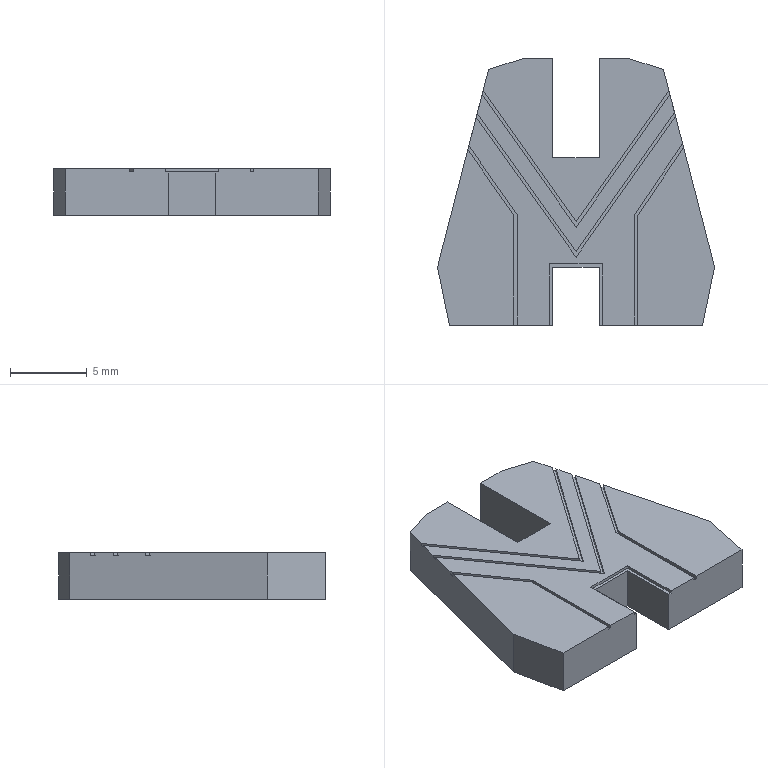Part | SolidWorks | features BaseBody 1 | 1 solid | 46 faces | box 17.999 x 17.317 x 3 mm | volume 684.94 mm3 | plane 46
STEP:
#1=CARTESIAN_POINT('',(-14.088,-24.638,1.3));
#2=VERTEX_POINT('',#1);
#3=CARTESIAN_POINT('',(-14.088,-20.86,1.3));
#4=VERTEX_POINT('',#3);
#5=CARTESIAN_POINT('',(-14.088,-24.638,1.3));
#6=DIRECTION('',(0.,1.,0.));
#7=VECTOR('',#6,1000.);
#8=LINE('',#5,#7);
#9=EDGE_CURVE('',#2,#4,#8,.T.);
#10=ORIENTED_EDGE('',*,*,#9,.T.);
#11=CARTESIAN_POINT('',(-14.088,-20.86,-1.5));
#12=VERTEX_POINT('',#11);
#13=CARTESIAN_POINT('',(-14.088,-20.86,-1.5));
#14=DIRECTION('',(0.,0.,1.));
#15=VECTOR('',#14,1000.);
#16=LINE('',#13,#15);
#17=EDGE_CURVE('',#12,#4,#16,.T.);
#18=ORIENTED_EDGE('',*,*,#17,.F.);
#19=CARTESIAN_POINT('',(-14.088,-24.638,-1.5));
#20=VERTEX_POINT('',#19);
#21=CARTESIAN_POINT('',(-14.088,-20.86,-1.5));
#22=DIRECTION('',(0.,1.,0.));
#23=VECTOR('',#22,1000.);
#24=LINE('',#21,#23);
#25=EDGE_CURVE('',#20,#12,#24,.T.);
#26=ORIENTED_EDGE('',*,*,#25,.F.);
#27=CARTESIAN_POINT('',(-14.088,-24.638,-1.5));
#28=DIRECTION('',(0.,0.,1.));
#29=VECTOR('',#28,1000.);
#30=LINE('',#27,#29);
#31=EDGE_CURVE('',#20,#2,#30,.T.);
#32=ORIENTED_EDGE('',*,*,#31,.T.);
#33=EDGE_LOOP('',(#10,#18,#26,#32));
#34=FACE_OUTER_BOUND('',#33,.T.);
#35=CARTESIAN_POINT('',(-14.088,-20.86,-1.5));
#36=DIRECTION('',(1.,0.,0.));
#37=DIRECTION('',(0.,1.,0.));
#38=AXIS2_PLACEMENT_3D('',#35,#36,#37);
#39=PLANE('',#38);
#40=ADVANCED_FACE('',(#34),#39,.F.);
#41=CARTESIAN_POINT('',(-17.085,-20.86,1.3));
#42=VERTEX_POINT('',#41);
#43=CARTESIAN_POINT('',(-14.088,-20.86,1.3));
#44=DIRECTION('',(-1.,0.,0.));
#45=VECTOR('',#44,1000.);
#46=LINE('',#43,#45);
#47=EDGE_CURVE('',#4,#42,#46,.T.);
#48=ORIENTED_EDGE('',*,*,#47,.T.);
#49=CARTESIAN_POINT('',(-17.085,-20.86,-1.5));
#50=VERTEX_POINT('',#49);
#51=CARTESIAN_POINT('',(-17.085,-20.86,-1.5));
#52=DIRECTION('',(0.,0.,1.));
#53=VECTOR('',#52,1000.);
#54=LINE('',#51,#53);
#55=EDGE_CURVE('',#50,#42,#54,.T.);
#56=ORIENTED_EDGE('',*,*,#55,.F.);
#57=CARTESIAN_POINT('',(-17.085,-20.86,-1.5));
#58=DIRECTION('',(-1.,0.,0.));
#59=VECTOR('',#58,1000.);
#60=LINE('',#57,#59);
#61=EDGE_CURVE('',#12,#50,#60,.T.);
#62=ORIENTED_EDGE('',*,*,#61,.F.);
#63=ORIENTED_EDGE('',*,*,#17,.T.);
#64=EDGE_LOOP('',(#48,#56,#62,#63));
#65=FACE_OUTER_BOUND('',#64,.T.);
#66=CARTESIAN_POINT('',(-17.085,-20.86,-1.5));
#67=DIRECTION('',(0.,1.,0.));
#68=DIRECTION('',(1.,0.,0.));
#69=AXIS2_PLACEMENT_3D('',#66,#67,#68);
#70=PLANE('',#69);
#71=ADVANCED_FACE('',(#65),#70,.F.);
#72=CARTESIAN_POINT('',(-17.085,-24.638,1.3));
#73=VERTEX_POINT('',#72);
#74=CARTESIAN_POINT('',(-17.085,-20.86,1.3));
#75=DIRECTION('',(0.,-1.,0.));
#76=VECTOR('',#75,1000.);
#77=LINE('',#74,#76);
#78=EDGE_CURVE('',#42,#73,#77,.T.);
#79=ORIENTED_EDGE('',*,*,#78,.T.);
#80=CARTESIAN_POINT('',(-17.085,-24.638,-1.5));
#81=VERTEX_POINT('',#80);
#82=CARTESIAN_POINT('',(-17.085,-24.638,-1.5));
#83=DIRECTION('',(0.,0.,1.));
#84=VECTOR('',#83,1000.);
#85=LINE('',#82,#84);
#86=EDGE_CURVE('',#81,#73,#85,.T.);
#87=ORIENTED_EDGE('',*,*,#86,.F.);
#88=CARTESIAN_POINT('',(-17.085,-20.86,-1.5));
#89=DIRECTION('',(0.,-1.,0.));
#90=VECTOR('',#89,1000.);
#91=LINE('',#88,#90);
#92=EDGE_CURVE('',#50,#81,#91,.T.);
#93=ORIENTED_EDGE('',*,*,#92,.F.);
#94=ORIENTED_EDGE('',*,*,#55,.T.);
#95=EDGE_LOOP('',(#79,#87,#93,#94));
#96=FACE_OUTER_BOUND('',#95,.T.);
#97=CARTESIAN_POINT('',(-17.085,-20.86,-1.5));
#98=DIRECTION('',(-1.,0.,0.));
#99=DIRECTION('',(0.,0.,1.));
#100=AXIS2_PLACEMENT_3D('',#97,#98,#99);
#101=PLANE('',#100);
#102=ADVANCED_FACE('',(#96),#101,.F.);
#103=CARTESIAN_POINT('',(-9.549,-9.394,1.3));
#104=VERTEX_POINT('',#103);
#105=CARTESIAN_POINT('',(-9.549,-9.394,1.5));
#106=VERTEX_POINT('',#105);
#107=CARTESIAN_POINT('',(-9.549,-9.394,1.5));
#108=DIRECTION('',(0.,0.,1.));
#109=VECTOR('',#108,1000.);
#110=LINE('',#107,#109);
#111=EDGE_CURVE('',#104,#106,#110,.T.);
#112=ORIENTED_EDGE('',*,*,#111,.T.);
#113=CARTESIAN_POINT('',(-15.575,-17.919,1.5));
#114=VERTEX_POINT('',#113);
#115=CARTESIAN_POINT('',(-15.575,-17.919,1.5));
#116=DIRECTION('',(0.5772,0.8166,0.));
#117=VECTOR('',#116,1000.);
#118=LINE('',#115,#117);
#119=EDGE_CURVE('',#114,#106,#118,.T.);
#120=ORIENTED_EDGE('',*,*,#119,.F.);
#121=CARTESIAN_POINT('',(-15.575,-17.919,1.3));
#122=VERTEX_POINT('',#121);
#123=CARTESIAN_POINT('',(-15.575,-17.919,1.3));
#124=DIRECTION('',(0.,0.,1.));
#125=VECTOR('',#124,1000.);
#126=LINE('',#123,#125);
#127=EDGE_CURVE('',#122,#114,#126,.T.);
#128=ORIENTED_EDGE('',*,*,#127,.F.);
#129=CARTESIAN_POINT('',(-15.575,-17.919,1.3));
#130=DIRECTION('',(0.5772,0.8166,0.));
#131=VECTOR('',#130,1000.);
#132=LINE('',#129,#131);
#133=EDGE_CURVE('',#122,#104,#132,.T.);
#134=ORIENTED_EDGE('',*,*,#133,.T.);
#135=EDGE_LOOP('',(#112,#120,#128,#134));
#136=FACE_OUTER_BOUND('',#135,.T.);
#137=CARTESIAN_POINT('',(-15.575,-17.919,1.3));
#138=DIRECTION('',(0.8166,-0.5772,0.));
#139=DIRECTION('',(0.,0.,-1.));
#140=AXIS2_PLACEMENT_3D('',#137,#138,#139);
#141=PLANE('',#140);
#142=ADVANCED_FACE('',(#136),#141,.T.);
#143=CARTESIAN_POINT('',(-21.62,-9.389,1.5));
#144=VERTEX_POINT('',#143);
#145=CARTESIAN_POINT('',(-21.62,-9.389,1.3));
#146=VERTEX_POINT('',#145);
#147=CARTESIAN_POINT('',(-21.62,-9.389,1.5));
#148=DIRECTION('',(0.,0.,-1.));
#149=VECTOR('',#148,1000.);
#150=LINE('',#147,#149);
#151=EDGE_CURVE('',#144,#146,#150,.T.);
#152=ORIENTED_EDGE('',*,*,#151,.T.);
#153=CARTESIAN_POINT('',(-22.587,-8.024,1.3));
#154=DIRECTION('',(0.5782,-0.8159,0.));
#155=VECTOR('',#154,1000.);
#156=LINE('',#153,#155);
#157=EDGE_CURVE('',#146,#122,#156,.T.);
#158=ORIENTED_EDGE('',*,*,#157,.T.);
#159=ORIENTED_EDGE('',*,*,#127,.T.);
#160=CARTESIAN_POINT('',(-18.822,-13.338,1.5));
#161=DIRECTION('',(-0.5782,0.8159,0.));
#162=VECTOR('',#161,1000.);
#163=LINE('',#160,#162);
#164=EDGE_CURVE('',#114,#144,#163,.T.);
#165=ORIENTED_EDGE('',*,*,#164,.T.);
#166=EDGE_LOOP('',(#152,#158,#159,#165));
#167=FACE_OUTER_BOUND('',#166,.T.);
#168=CARTESIAN_POINT('',(-22.587,-8.024,1.3));
#169=DIRECTION('',(-0.8159,-0.5782,0.));
#170=DIRECTION('',(-0.5782,0.8159,0.));
#171=AXIS2_PLACEMENT_3D('',#168,#169,#170);
#172=PLANE('',#171);
#173=ADVANCED_FACE('',(#167),#172,.T.);
#174=CARTESIAN_POINT('',(-15.575,-18.266,1.5));
#175=VERTEX_POINT('',#174);
#176=CARTESIAN_POINT('',(-21.686,-9.642,1.5));
#177=VERTEX_POINT('',#176);
#178=CARTESIAN_POINT('',(-18.985,-13.453,1.5));
#179=DIRECTION('',(-0.5782,0.8159,0.));
#180=VECTOR('',#179,1000.);
#181=LINE('',#178,#180);
#182=EDGE_CURVE('',#175,#177,#181,.T.);
#183=ORIENTED_EDGE('',*,*,#182,.F.);
#184=CARTESIAN_POINT('',(-15.575,-18.266,1.3));
#185=VERTEX_POINT('',#184);
#186=CARTESIAN_POINT('',(-15.575,-18.266,1.3));
#187=DIRECTION('',(0.,0.,1.));
#188=VECTOR('',#187,1000.);
#189=LINE('',#186,#188);
#190=EDGE_CURVE('',#185,#175,#189,.T.);
#191=ORIENTED_EDGE('',*,*,#190,.F.);
#192=CARTESIAN_POINT('',(-21.686,-9.642,1.3));
#193=VERTEX_POINT('',#192);
#194=CARTESIAN_POINT('',(-22.75,-8.14,1.3));
#195=DIRECTION('',(0.5782,-0.8159,0.));
#196=VECTOR('',#195,1000.);
#197=LINE('',#194,#196);
#198=EDGE_CURVE('',#193,#185,#197,.T.);
#199=ORIENTED_EDGE('',*,*,#198,.F.);
#200=CARTESIAN_POINT('',(-21.686,-9.642,1.5));
#201=DIRECTION('',(0.,0.,-1.));
#202=VECTOR('',#201,1000.);
#203=LINE('',#200,#202);
#204=EDGE_CURVE('',#177,#193,#203,.T.);
#205=ORIENTED_EDGE('',*,*,#204,.F.);
#206=EDGE_LOOP('',(#183,#191,#199,#205));
#207=FACE_OUTER_BOUND('',#206,.T.);
#208=CARTESIAN_POINT('',(-22.75,-8.14,1.3));
#209=DIRECTION('',(-0.8159,-0.5782,0.));
#210=DIRECTION('',(-0.5782,0.8159,0.));
#211=AXIS2_PLACEMENT_3D('',#208,#209,#210);
#212=PLANE('',#211);
#213=ADVANCED_FACE('',(#207),#212,.F.);
#214=CARTESIAN_POINT('',(-9.484,-9.648,1.3));
#215=VERTEX_POINT('',#214);
#216=CARTESIAN_POINT('',(-15.412,-18.035,1.3));
#217=DIRECTION('',(0.5772,0.8166,0.));
#218=VECTOR('',#217,1000.);
#219=LINE('',#216,#218);
#220=EDGE_CURVE('',#185,#215,#219,.T.);
#221=ORIENTED_EDGE('',*,*,#220,.F.);
#222=ORIENTED_EDGE('',*,*,#190,.T.);
#223=CARTESIAN_POINT('',(-9.484,-9.648,1.5));
#224=VERTEX_POINT('',#223);
#225=CARTESIAN_POINT('',(-15.412,-18.035,1.5));
#226=DIRECTION('',(0.5772,0.8166,0.));
#227=VECTOR('',#226,1000.);
#228=LINE('',#225,#227);
#229=EDGE_CURVE('',#175,#224,#228,.T.);
#230=ORIENTED_EDGE('',*,*,#229,.T.);
#231=CARTESIAN_POINT('',(-9.484,-9.648,1.5));
#232=DIRECTION('',(0.,0.,1.));
#233=VECTOR('',#232,1000.);
#234=LINE('',#231,#233);
#235=EDGE_CURVE('',#215,#224,#234,.T.);
#236=ORIENTED_EDGE('',*,*,#235,.F.);
#237=EDGE_LOOP('',(#221,#222,#230,#236));
#238=FACE_OUTER_BOUND('',#237,.T.);
#239=CARTESIAN_POINT('',(-15.412,-18.035,1.3));
#240=DIRECTION('',(0.8166,-0.5772,0.));
#241=DIRECTION('',(0.,0.,-1.));
#242=AXIS2_PLACEMENT_3D('',#239,#240,#241);
#243=PLANE('',#242);
#244=ADVANCED_FACE('',(#238),#243,.F.);
#245=ORIENTED_EDGE('',*,*,#198,.T.);
#246=ORIENTED_EDGE('',*,*,#220,.T.);
#247=CARTESIAN_POINT('',(-9.904,-8.023,1.3));
#248=DIRECTION('',(0.2503,-0.9682,0.));
#249=VECTOR('',#248,1000.);
#250=LINE('',#247,#249);
#251=EDGE_CURVE('',#104,#215,#250,.T.);
#252=ORIENTED_EDGE('',*,*,#251,.F.);
#253=ORIENTED_EDGE('',*,*,#133,.F.);
#254=ORIENTED_EDGE('',*,*,#157,.F.);
#255=CARTESIAN_POINT('',(-24.585,-20.858,1.3));
#256=DIRECTION('',(0.2503,0.9682,0.));
#257=VECTOR('',#256,1000.);
#258=LINE('',#255,#257);
#259=EDGE_CURVE('',#193,#146,#258,.T.);
#260=ORIENTED_EDGE('',*,*,#259,.F.);
#261=EDGE_LOOP('',(#245,#246,#252,#253,#254,#260));
#262=FACE_OUTER_BOUND('',#261,.T.);
#263=CARTESIAN_POINT('',(0.,0.,1.3));
#264=DIRECTION('',(0.,0.,-1.));
#265=DIRECTION('',(0.,-1.,0.));
#266=AXIS2_PLACEMENT_3D('',#263,#264,#265);
#267=PLANE('',#266);
#268=ADVANCED_FACE('',(#262),#267,.F.);
#269=CARTESIAN_POINT('',(-17.285,-20.66,1.3));
#270=VERTEX_POINT('',#269);
#271=CARTESIAN_POINT('',(-17.285,-24.638,1.3));
#272=VERTEX_POINT('',#271);
#273=CARTESIAN_POINT('',(-17.285,-20.86,1.3));
#274=DIRECTION('',(0.,-1.,0.));
#275=VECTOR('',#274,1000.);
#276=LINE('',#273,#275);
#277=EDGE_CURVE('',#270,#272,#276,.T.);
#278=ORIENTED_EDGE('',*,*,#277,.T.);
#279=CARTESIAN_POINT('',(-17.085,-24.638,1.3));
#280=DIRECTION('',(-1.,0.,0.));
#281=VECTOR('',#280,1000.);
#282=LINE('',#279,#281);
#283=EDGE_CURVE('',#73,#272,#282,.T.);
#284=ORIENTED_EDGE('',*,*,#283,.F.);
#285=ORIENTED_EDGE('',*,*,#78,.F.);
#286=ORIENTED_EDGE('',*,*,#47,.F.);
#287=ORIENTED_EDGE('',*,*,#9,.F.);
#288=CARTESIAN_POINT('',(-13.888,-24.638,1.3));
#289=VERTEX_POINT('',#288);
#290=CARTESIAN_POINT('',(-13.888,-24.638,1.3));
#291=DIRECTION('',(-1.,0.,0.));
#292=VECTOR('',#291,1000.);
#293=LINE('',#290,#292);
#294=EDGE_CURVE('',#289,#2,#293,.T.);
#295=ORIENTED_EDGE('',*,*,#294,.F.);
#296=CARTESIAN_POINT('',(-13.888,-20.66,1.3));
#297=VERTEX_POINT('',#296);
#298=CARTESIAN_POINT('',(-13.888,-24.638,1.3));
#299=DIRECTION('',(0.,1.,0.));
#300=VECTOR('',#299,1000.);
#301=LINE('',#298,#300);
#302=EDGE_CURVE('',#289,#297,#301,.T.);
#303=ORIENTED_EDGE('',*,*,#302,.T.);
#304=CARTESIAN_POINT('',(-14.088,-20.66,1.3));
#305=DIRECTION('',(-1.,0.,0.));
#306=VECTOR('',#305,1000.);
#307=LINE('',#304,#306);
#308=EDGE_CURVE('',#297,#270,#307,.T.);
#309=ORIENTED_EDGE('',*,*,#308,.T.);
#310=EDGE_LOOP('',(#278,#284,#285,#286,#287,#295,#303,#309));
#311=FACE_OUTER_BOUND('',#310,.T.);
#312=CARTESIAN_POINT('',(0.,0.,1.3));
#313=DIRECTION('',(0.,0.,1.));
#314=DIRECTION('',(1.,0.,0.));
#315=AXIS2_PLACEMENT_3D('',#312,#313,#314);
#316=PLANE('',#315);
#317=ADVANCED_FACE('',(#311),#316,.T.);
#318=CARTESIAN_POINT('',(-13.888,-24.638,1.5));
#319=VERTEX_POINT('',#318);
#320=CARTESIAN_POINT('',(-13.888,-20.66,1.5));
#321=VERTEX_POINT('',#320);
#322=CARTESIAN_POINT('',(-13.888,-24.638,1.5));
#323=DIRECTION('',(0.,1.,0.));
#324=VECTOR('',#323,1000.);
#325=LINE('',#322,#324);
#326=EDGE_CURVE('',#319,#321,#325,.T.);
#327=ORIENTED_EDGE('',*,*,#326,.T.);
#328=CARTESIAN_POINT('',(-13.888,-20.66,1.3));
#329=DIRECTION('',(0.,0.,1.));
#330=VECTOR('',#329,1000.);
#331=LINE('',#328,#330);
#332=EDGE_CURVE('',#297,#321,#331,.T.);
#333=ORIENTED_EDGE('',*,*,#332,.F.);
#334=ORIENTED_EDGE('',*,*,#302,.F.);
#335=CARTESIAN_POINT('',(-13.888,-24.638,1.3));
#336=DIRECTION('',(0.,0.,1.));
#337=VECTOR('',#336,1000.);
#338=LINE('',#335,#337);
#339=EDGE_CURVE('',#289,#319,#338,.T.);
#340=ORIENTED_EDGE('',*,*,#339,.T.);
#341=EDGE_LOOP('',(#327,#333,#334,#340));
#342=FACE_OUTER_BOUND('',#341,.T.);
#343=CARTESIAN_POINT('',(-13.888,-24.638,1.3));
#344=DIRECTION('',(1.,0.,0.));
#345=DIRECTION('',(0.,1.,0.));
#346=AXIS2_PLACEMENT_3D('',#343,#344,#345);
#347=PLANE('',#346);
#348=ADVANCED_FACE('',(#342),#347,.F.);
#349=CARTESIAN_POINT('',(-17.285,-20.66,1.5));
#350=VERTEX_POINT('',#349);
#351=CARTESIAN_POINT('',(-14.088,-20.66,1.5));
#352=DIRECTION('',(-1.,0.,0.));
#353=VECTOR('',#352,1000.);
#354=LINE('',#351,#353);
#355=EDGE_CURVE('',#321,#350,#354,.T.);
#356=ORIENTED_EDGE('',*,*,#355,.T.);
#357=CARTESIAN_POINT('',(-17.285,-20.66,1.3));
#358=DIRECTION('',(0.,0.,1.));
#359=VECTOR('',#358,1000.);
#360=LINE('',#357,#359);
#361=EDGE_CURVE('',#270,#350,#360,.T.);
#362=ORIENTED_EDGE('',*,*,#361,.F.);
#363=ORIENTED_EDGE('',*,*,#308,.F.);
#364=ORIENTED_EDGE('',*,*,#332,.T.);
#365=EDGE_LOOP('',(#356,#362,#363,#364));
#366=FACE_OUTER_BOUND('',#365,.T.);
#367=CARTESIAN_POINT('',(-14.088,-20.66,1.3));
#368=DIRECTION('',(0.,1.,0.));
#369=DIRECTION('',(1.,0.,0.));
#370=AXIS2_PLACEMENT_3D('',#367,#368,#369);
#371=PLANE('',#370);
#372=ADVANCED_FACE('',(#366),#371,.F.);
#373=CARTESIAN_POINT('',(-17.285,-24.638,1.5));
#374=VERTEX_POINT('',#373);
#375=CARTESIAN_POINT('',(-17.285,-20.86,1.5));
#376=DIRECTION('',(0.,-1.,0.));
#377=VECTOR('',#376,1000.);
#378=LINE('',#375,#377);
#379=EDGE_CURVE('',#350,#374,#378,.T.);
#380=ORIENTED_EDGE('',*,*,#379,.T.);
#381=CARTESIAN_POINT('',(-17.285,-24.638,1.3));
#382=DIRECTION('',(0.,0.,1.));
#383=VECTOR('',#382,1000.);
#384=LINE('',#381,#383);
#385=EDGE_CURVE('',#272,#374,#384,.T.);
#386=ORIENTED_EDGE('',*,*,#385,.F.);
#387=ORIENTED_EDGE('',*,*,#277,.F.);
#388=ORIENTED_EDGE('',*,*,#361,.T.);
#389=EDGE_LOOP('',(#380,#386,#387,#388));
#390=FACE_OUTER_BOUND('',#389,.T.);
#391=CARTESIAN_POINT('',(-17.285,-20.86,1.3));
#392=DIRECTION('',(-1.,0.,0.));
#393=DIRECTION('',(0.,0.,1.));
#394=AXIS2_PLACEMENT_3D('',#391,#392,#393);
#395=PLANE('',#394);
#396=ADVANCED_FACE('',(#390),#395,.F.);
#397=CARTESIAN_POINT('',(-11.773,-24.638,1.5));
#398=VERTEX_POINT('',#397);
#399=CARTESIAN_POINT('',(-11.773,-24.63,1.5));
#400=VERTEX_POINT('',#399);
#401=CARTESIAN_POINT('',(-11.773,-24.638,1.5));
#402=CARTESIAN_POINT('',(-11.773,-24.633,1.5));
#403=CARTESIAN_POINT('',(-11.773,-24.63,1.5));
#404=B_SPLINE_CURVE_WITH_KNOTS('',2,(#401,#402,#403),.UNSPECIFIED.,.F.,.F.,(3,3),(0.05762,0.05882),.UNSPECIFIED.);
#405=EDGE_CURVE('',#398,#400,#404,.T.);
#406=ORIENTED_EDGE('',*,*,#405,.F.);
#407=CARTESIAN_POINT('',(-11.773,-24.638,1.3));
#408=VERTEX_POINT('',#407);
#409=CARTESIAN_POINT('',(-11.773,-24.638,1.3));
#410=DIRECTION('',(0.,0.,1.));
#411=VECTOR('',#410,1000.);
#412=LINE('',#409,#411);
#413=EDGE_CURVE('',#408,#398,#412,.T.);
#414=ORIENTED_EDGE('',*,*,#413,.F.);
#415=CARTESIAN_POINT('',(-11.773,-24.63,1.3));
#416=VERTEX_POINT('',#415);
#417=CARTESIAN_POINT('',(-11.773,-24.638,1.3));
#418=CARTESIAN_POINT('',(-11.773,-24.633,1.3));
#419=CARTESIAN_POINT('',(-11.773,-24.63,1.3));
#420=B_SPLINE_CURVE_WITH_KNOTS('',2,(#417,#418,#419),.UNSPECIFIED.,.F.,.F.,(3,3),(0.05762,0.05882),.UNSPECIFIED.);
#421=EDGE_CURVE('',#408,#416,#420,.T.);
#422=ORIENTED_EDGE('',*,*,#421,.T.);
#423=CARTESIAN_POINT('',(-11.773,-17.448,1.3));
#424=VERTEX_POINT('',#423);
#425=CARTESIAN_POINT('',(-11.773,-24.63,1.3));
#426=DIRECTION('',(0.,1.,0.));
#427=VECTOR('',#426,1000.);
#428=LINE('',#425,#427);
#429=EDGE_CURVE('',#416,#424,#428,.T.);
#430=ORIENTED_EDGE('',*,*,#429,.T.);
#431=CARTESIAN_POINT('',(-11.773,-17.448,1.5));
#432=VERTEX_POINT('',#431);
#433=CARTESIAN_POINT('',(-11.773,-17.448,1.3));
#434=DIRECTION('',(0.,0.,1.));
#435=VECTOR('',#434,1000.);
#436=LINE('',#433,#435);
#437=EDGE_CURVE('',#424,#432,#436,.T.);
#438=ORIENTED_EDGE('',*,*,#437,.T.);
#439=CARTESIAN_POINT('',(-11.773,-24.63,1.5));
#440=DIRECTION('',(0.,1.,0.));
#441=VECTOR('',#440,1000.);
#442=LINE('',#439,#441);
#443=EDGE_CURVE('',#400,#432,#442,.T.);
#444=ORIENTED_EDGE('',*,*,#443,.F.);
#445=EDGE_LOOP('',(#406,#414,#422,#430,#438,#444));
#446=FACE_OUTER_BOUND('',#445,.T.);
#447=CARTESIAN_POINT('',(-11.773,-24.638,1.3));
#448=DIRECTION('',(1.,0.,0.));
#449=DIRECTION('',(0.,1.,0.));
#450=AXIS2_PLACEMENT_3D('',#447,#448,#449);
#451=PLANE('',#450);
#452=ADVANCED_FACE('',(#446),#451,.T.);
#453=CARTESIAN_POINT('',(-11.573,-24.638,1.5));
#454=VERTEX_POINT('',#453);
#455=CARTESIAN_POINT('',(-11.573,-17.509,1.5));
#456=VERTEX_POINT('',#455);
#457=CARTESIAN_POINT('',(-11.573,-24.63,1.5));
#458=DIRECTION('',(0.,1.,0.));
#459=VECTOR('',#458,1000.);
#460=LINE('',#457,#459);
#461=EDGE_CURVE('',#454,#456,#460,.T.);
#462=ORIENTED_EDGE('',*,*,#461,.T.);
#463=CARTESIAN_POINT('',(-11.573,-17.509,1.3));
#464=VERTEX_POINT('',#463);
#465=CARTESIAN_POINT('',(-11.573,-17.509,1.3));
#466=DIRECTION('',(0.,0.,1.));
#467=VECTOR('',#466,1000.);
#468=LINE('',#465,#467);
#469=EDGE_CURVE('',#464,#456,#468,.T.);
#470=ORIENTED_EDGE('',*,*,#469,.F.);
#471=CARTESIAN_POINT('',(-11.573,-24.638,1.3));
#472=VERTEX_POINT('',#471);
#473=CARTESIAN_POINT('',(-11.573,-24.638,1.3));
#474=DIRECTION('',(0.,1.,0.));
#475=VECTOR('',#474,1000.);
#476=LINE('',#473,#475);
#477=EDGE_CURVE('',#472,#464,#476,.T.);
#478=ORIENTED_EDGE('',*,*,#477,.F.);
#479=CARTESIAN_POINT('',(-11.573,-24.638,1.3));
#480=DIRECTION('',(0.,0.,1.));
#481=VECTOR('',#480,1000.);
#482=LINE('',#479,#481);
#483=EDGE_CURVE('',#472,#454,#482,.T.);
#484=ORIENTED_EDGE('',*,*,#483,.T.);
#485=EDGE_LOOP('',(#462,#470,#478,#484));
#486=FACE_OUTER_BOUND('',#485,.T.);
#487=CARTESIAN_POINT('',(-11.573,-24.63,1.3));
#488=DIRECTION('',(1.,0.,0.));
#489=DIRECTION('',(0.,1.,0.));
#490=AXIS2_PLACEMENT_3D('',#487,#488,#489);
#491=PLANE('',#490);
#492=ADVANCED_FACE('',(#486),#491,.F.);
#493=CARTESIAN_POINT('',(-8.658,-12.841,1.3));
#494=VERTEX_POINT('',#493);
#495=CARTESIAN_POINT('',(-8.658,-12.841,1.5));
#496=VERTEX_POINT('',#495);
#497=CARTESIAN_POINT('',(-8.658,-12.841,1.5));
#498=DIRECTION('',(0.,0.,1.));
#499=VECTOR('',#498,1000.);
#500=LINE('',#497,#499);
#501=EDGE_CURVE('',#494,#496,#500,.T.);
#502=ORIENTED_EDGE('',*,*,#501,.T.);
#503=CARTESIAN_POINT('',(-11.773,-17.448,1.5));
#504=DIRECTION('',(0.5601,0.8284,0.));
#505=VECTOR('',#504,1000.);
#506=LINE('',#503,#505);
#507=EDGE_CURVE('',#432,#496,#506,.T.);
#508=ORIENTED_EDGE('',*,*,#507,.F.);
#509=ORIENTED_EDGE('',*,*,#437,.F.);
#510=CARTESIAN_POINT('',(-11.773,-17.448,1.3));
#511=DIRECTION('',(0.5601,0.8284,0.));
#512=VECTOR('',#511,1000.);
#513=LINE('',#510,#512);
#514=EDGE_CURVE('',#424,#494,#513,.T.);
#515=ORIENTED_EDGE('',*,*,#514,.T.);
#516=EDGE_LOOP('',(#502,#508,#509,#515));
#517=FACE_OUTER_BOUND('',#516,.T.);
#518=CARTESIAN_POINT('',(-11.773,-17.448,1.3));
#519=DIRECTION('',(0.8284,-0.5601,0.));
#520=DIRECTION('',(0.,0.,-1.));
#521=AXIS2_PLACEMENT_3D('',#518,#519,#520);
#522=PLANE('',#521);
#523=ADVANCED_FACE('',(#517),#522,.T.);
#524=CARTESIAN_POINT('',(-8.591,-13.099,1.3));
#525=VERTEX_POINT('',#524);
#526=CARTESIAN_POINT('',(-11.607,-17.56,1.3));
#527=DIRECTION('',(0.5601,0.8284,0.));
#528=VECTOR('',#527,1000.);
#529=LINE('',#526,#528);
#530=EDGE_CURVE('',#464,#525,#529,.T.);
#531=ORIENTED_EDGE('',*,*,#530,.F.);
#532=ORIENTED_EDGE('',*,*,#469,.T.);
#533=CARTESIAN_POINT('',(-8.591,-13.099,1.5));
#534=VERTEX_POINT('',#533);
#535=CARTESIAN_POINT('',(-11.607,-17.56,1.5));
#536=DIRECTION('',(0.5601,0.8284,0.));
#537=VECTOR('',#536,1000.);
#538=LINE('',#535,#537);
#539=EDGE_CURVE('',#456,#534,#538,.T.);
#540=ORIENTED_EDGE('',*,*,#539,.T.);
#541=CARTESIAN_POINT('',(-8.591,-13.099,1.5));
#542=DIRECTION('',(0.,0.,1.));
#543=VECTOR('',#542,1000.);
#544=LINE('',#541,#543);
#545=EDGE_CURVE('',#525,#534,#544,.T.);
#546=ORIENTED_EDGE('',*,*,#545,.F.);
#547=EDGE_LOOP('',(#531,#532,#540,#546));
#548=FACE_OUTER_BOUND('',#547,.T.);
#549=CARTESIAN_POINT('',(-11.607,-17.56,1.3));
#550=DIRECTION('',(0.8284,-0.5601,0.));
#551=DIRECTION('',(0.,0.,-1.));
#552=AXIS2_PLACEMENT_3D('',#549,#550,#551);
#553=PLANE('',#552);
#554=ADVANCED_FACE('',(#548),#553,.F.);
#555=CARTESIAN_POINT('',(-9.904,-8.023,1.3));
#556=DIRECTION('',(-0.2503,0.9682,0.));
#557=VECTOR('',#556,1000.);
#558=LINE('',#555,#557);
#559=EDGE_CURVE('',#525,#494,#558,.T.);
#560=ORIENTED_EDGE('',*,*,#559,.T.);
#561=ORIENTED_EDGE('',*,*,#514,.F.);
#562=ORIENTED_EDGE('',*,*,#429,.F.);
#563=ORIENTED_EDGE('',*,*,#421,.F.);
#564=CARTESIAN_POINT('',(-11.573,-24.638,1.3));
#565=DIRECTION('',(-1.,0.,0.));
#566=VECTOR('',#565,1000.);
#567=LINE('',#564,#566);
#568=EDGE_CURVE('',#472,#408,#567,.T.);
#569=ORIENTED_EDGE('',*,*,#568,.F.);
#570=ORIENTED_EDGE('',*,*,#477,.T.);
#571=ORIENTED_EDGE('',*,*,#530,.T.);
#572=EDGE_LOOP('',(#560,#561,#562,#563,#569,#570,#571));
#573=FACE_OUTER_BOUND('',#572,.T.);
#574=CARTESIAN_POINT('',(-19.615,-24.63,1.3));
#575=DIRECTION('',(0.,0.,1.));
#576=DIRECTION('',(1.,0.,0.));
#577=AXIS2_PLACEMENT_3D('',#574,#575,#576);
#578=PLANE('',#577);
#579=ADVANCED_FACE('',(#573),#578,.T.);
#580=CARTESIAN_POINT('',(-22.006,-10.879,1.3));
#581=VERTEX_POINT('',#580);
#582=CARTESIAN_POINT('',(-22.071,-11.132,1.3));
#583=VERTEX_POINT('',#582);
#584=CARTESIAN_POINT('',(-24.585,-20.858,1.3));
#585=DIRECTION('',(-0.2503,-0.9682,0.));
#586=VECTOR('',#585,1000.);
#587=LINE('',#584,#586);
#588=EDGE_CURVE('',#581,#583,#587,.T.);
#589=ORIENTED_EDGE('',*,*,#588,.T.);
#590=CARTESIAN_POINT('',(-15.583,-20.21,1.3));
#591=VERTEX_POINT('',#590);
#592=CARTESIAN_POINT('',(-15.583,-20.21,1.3));
#593=DIRECTION('',(-0.5815,0.8136,0.));
#594=VECTOR('',#593,1000.);
#595=LINE('',#592,#594);
#596=EDGE_CURVE('',#591,#583,#595,.T.);
#597=ORIENTED_EDGE('',*,*,#596,.F.);
#598=CARTESIAN_POINT('',(-9.119,-11.059,1.3));
#599=VERTEX_POINT('',#598);
#600=CARTESIAN_POINT('',(-8.282,-9.873,1.3));
#601=DIRECTION('',(-0.5769,-0.8168,0.));
#602=VECTOR('',#601,1000.);
#603=LINE('',#600,#602);
#604=EDGE_CURVE('',#599,#591,#603,.T.);
#605=ORIENTED_EDGE('',*,*,#604,.F.);
#606=CARTESIAN_POINT('',(-9.185,-10.805,1.3));
#607=VERTEX_POINT('',#606);
#608=CARTESIAN_POINT('',(-9.904,-8.023,1.3));
#609=DIRECTION('',(-0.2503,0.9682,0.));
#610=VECTOR('',#609,1000.);
#611=LINE('',#608,#610);
#612=EDGE_CURVE('',#599,#607,#611,.T.);
#613=ORIENTED_EDGE('',*,*,#612,.T.);
#614=CARTESIAN_POINT('',(-15.584,-19.865,1.3));
#615=VERTEX_POINT('',#614);
#616=CARTESIAN_POINT('',(-8.445,-9.758,1.3));
#617=DIRECTION('',(-0.5769,-0.8168,0.));
#618=VECTOR('',#617,1000.);
#619=LINE('',#616,#618);
#620=EDGE_CURVE('',#607,#615,#619,.T.);
#621=ORIENTED_EDGE('',*,*,#620,.T.);
#622=CARTESIAN_POINT('',(-15.42,-20.094,1.3));
#623=DIRECTION('',(-0.5815,0.8136,0.));
#624=VECTOR('',#623,1000.);
#625=LINE('',#622,#624);
#626=EDGE_CURVE('',#615,#581,#625,.T.);
#627=ORIENTED_EDGE('',*,*,#626,.T.);
#628=EDGE_LOOP('',(#589,#597,#605,#613,#621,#627));
#629=FACE_OUTER_BOUND('',#628,.T.);
#630=CARTESIAN_POINT('',(-19.615,-24.63,1.3));
#631=DIRECTION('',(0.,0.,1.));
#632=DIRECTION('',(1.,0.,0.));
#633=AXIS2_PLACEMENT_3D('',#630,#631,#632);
#634=PLANE('',#633);
#635=ADVANCED_FACE('',(#629),#634,.T.);
#636=ORIENTED_EDGE('',*,*,#626,.F.);
#637=CARTESIAN_POINT('',(-15.584,-19.865,1.5));
#638=VERTEX_POINT('',#637);
#639=CARTESIAN_POINT('',(-15.584,-19.865,1.3));
#640=DIRECTION('',(0.,0.,1.));
#641=VECTOR('',#640,1000.);
#642=LINE('',#639,#641);
#643=EDGE_CURVE('',#615,#638,#642,.T.);
#644=ORIENTED_EDGE('',*,*,#643,.T.);
#645=CARTESIAN_POINT('',(-22.006,-10.879,1.5));
#646=VERTEX_POINT('',#645);
#647=CARTESIAN_POINT('',(-15.42,-20.094,1.5));
#648=DIRECTION('',(-0.5815,0.8136,0.));
#649=VECTOR('',#648,1000.);
#650=LINE('',#647,#649);
#651=EDGE_CURVE('',#638,#646,#650,.T.);
#652=ORIENTED_EDGE('',*,*,#651,.T.);
#653=CARTESIAN_POINT('',(-22.006,-10.879,1.5));
#654=DIRECTION('',(0.,0.,1.));
#655=VECTOR('',#654,1000.);
#656=LINE('',#653,#655);
#657=EDGE_CURVE('',#581,#646,#656,.T.);
#658=ORIENTED_EDGE('',*,*,#657,.F.);
#659=EDGE_LOOP('',(#636,#644,#652,#658));
#660=FACE_OUTER_BOUND('',#659,.T.);
#661=CARTESIAN_POINT('',(-15.42,-20.094,1.3));
#662=DIRECTION('',(0.8136,0.5815,0.));
#663=DIRECTION('',(0.,0.,-1.));
#664=AXIS2_PLACEMENT_3D('',#661,#662,#663);
#665=PLANE('',#664);
#666=ADVANCED_FACE('',(#660),#665,.F.);
#667=CARTESIAN_POINT('',(-9.185,-10.805,1.5));
#668=VERTEX_POINT('',#667);
#669=CARTESIAN_POINT('',(-1.036,0.7318,1.5));
#670=DIRECTION('',(0.5769,0.8168,0.));
#671=VECTOR('',#670,1000.);
#672=LINE('',#669,#671);
#673=EDGE_CURVE('',#638,#668,#672,.T.);
#674=ORIENTED_EDGE('',*,*,#673,.F.);
#675=ORIENTED_EDGE('',*,*,#643,.F.);
#676=ORIENTED_EDGE('',*,*,#620,.F.);
#677=CARTESIAN_POINT('',(-9.185,-10.805,1.5));
#678=DIRECTION('',(0.,0.,-1.));
#679=VECTOR('',#678,1000.);
#680=LINE('',#677,#679);
#681=EDGE_CURVE('',#668,#607,#680,.T.);
#682=ORIENTED_EDGE('',*,*,#681,.F.);
#683=EDGE_LOOP('',(#674,#675,#676,#682));
#684=FACE_OUTER_BOUND('',#683,.T.);
#685=CARTESIAN_POINT('',(-8.445,-9.758,1.3));
#686=DIRECTION('',(-0.8168,0.5769,0.));
#687=DIRECTION('',(0.,0.,1.));
#688=AXIS2_PLACEMENT_3D('',#685,#686,#687);
#689=PLANE('',#688);
#690=ADVANCED_FACE('',(#684),#689,.F.);
#691=CARTESIAN_POINT('',(-9.119,-11.059,1.5));
#692=VERTEX_POINT('',#691);
#693=CARTESIAN_POINT('',(-9.119,-11.059,1.5));
#694=DIRECTION('',(0.,0.,-1.));
#695=VECTOR('',#694,1000.);
#696=LINE('',#693,#695);
#697=EDGE_CURVE('',#692,#599,#696,.T.);
#698=ORIENTED_EDGE('',*,*,#697,.T.);
#699=ORIENTED_EDGE('',*,*,#604,.T.);
#700=CARTESIAN_POINT('',(-15.583,-20.21,1.5));
#701=VERTEX_POINT('',#700);
#702=CARTESIAN_POINT('',(-15.583,-20.21,1.3));
#703=DIRECTION('',(0.,0.,1.));
#704=VECTOR('',#703,1000.);
#705=LINE('',#702,#704);
#706=EDGE_CURVE('',#591,#701,#705,.T.);
#707=ORIENTED_EDGE('',*,*,#706,.T.);
#708=CARTESIAN_POINT('',(-0.8727,0.6164,1.5));
#709=DIRECTION('',(0.5769,0.8168,0.));
#710=VECTOR('',#709,1000.);
#711=LINE('',#708,#710);
#712=EDGE_CURVE('',#701,#692,#711,.T.);
#713=ORIENTED_EDGE('',*,*,#712,.T.);
#714=EDGE_LOOP('',(#698,#699,#707,#713));
#715=FACE_OUTER_BOUND('',#714,.T.);
#716=CARTESIAN_POINT('',(-8.282,-9.873,1.3));
#717=DIRECTION('',(-0.8168,0.5769,0.));
#718=DIRECTION('',(0.,0.,1.));
#719=AXIS2_PLACEMENT_3D('',#716,#717,#718);
#720=PLANE('',#719);
#721=ADVANCED_FACE('',(#715),#720,.T.);
#722=CARTESIAN_POINT('',(-22.071,-11.132,1.5));
#723=VERTEX_POINT('',#722);
#724=CARTESIAN_POINT('',(-22.071,-11.132,1.5));
#725=DIRECTION('',(0.,0.,1.));
#726=VECTOR('',#725,1000.);
#727=LINE('',#724,#726);
#728=EDGE_CURVE('',#583,#723,#727,.T.);
#729=ORIENTED_EDGE('',*,*,#728,.T.);
#730=CARTESIAN_POINT('',(-15.583,-20.21,1.5));
#731=DIRECTION('',(-0.5815,0.8136,0.));
#732=VECTOR('',#731,1000.);
#733=LINE('',#730,#732);
#734=EDGE_CURVE('',#701,#723,#733,.T.);
#735=ORIENTED_EDGE('',*,*,#734,.F.);
#736=ORIENTED_EDGE('',*,*,#706,.F.);
#737=ORIENTED_EDGE('',*,*,#596,.T.);
#738=EDGE_LOOP('',(#729,#735,#736,#737));
#739=FACE_OUTER_BOUND('',#738,.T.);
#740=CARTESIAN_POINT('',(-15.583,-20.21,1.3));
#741=DIRECTION('',(0.8136,0.5815,0.));
#742=DIRECTION('',(0.,0.,-1.));
#743=AXIS2_PLACEMENT_3D('',#740,#741,#742);
#744=PLANE('',#743);
#745=ADVANCED_FACE('',(#739),#744,.T.);
#746=CARTESIAN_POINT('',(-22.549,-12.982,1.3));
#747=VERTEX_POINT('',#746);
#748=CARTESIAN_POINT('',(-22.615,-13.236,1.3));
#749=VERTEX_POINT('',#748);
#750=CARTESIAN_POINT('',(-24.585,-20.858,1.3));
#751=DIRECTION('',(-0.2503,-0.9682,0.));
#752=VECTOR('',#751,1000.);
#753=LINE('',#750,#752);
#754=EDGE_CURVE('',#747,#749,#753,.T.);
#755=ORIENTED_EDGE('',*,*,#754,.T.);
#756=CARTESIAN_POINT('',(-19.615,-17.511,1.3));
#757=VERTEX_POINT('',#756);
#758=CARTESIAN_POINT('',(-23.67,-11.733,1.3));
#759=DIRECTION('',(0.5744,-0.8186,0.));
#760=VECTOR('',#759,1000.);
#761=LINE('',#758,#760);
#762=EDGE_CURVE('',#749,#757,#761,.T.);
#763=ORIENTED_EDGE('',*,*,#762,.T.);
#764=CARTESIAN_POINT('',(-19.615,-24.638,1.3));
#765=VERTEX_POINT('',#764);
#766=CARTESIAN_POINT('',(-19.615,-24.63,1.3));
#767=DIRECTION('',(0.,-1.,0.));
#768=VECTOR('',#767,1000.);
#769=LINE('',#766,#768);
#770=EDGE_CURVE('',#757,#765,#769,.T.);
#771=ORIENTED_EDGE('',*,*,#770,.T.);
#772=CARTESIAN_POINT('',(-19.415,-24.638,1.3));
#773=VERTEX_POINT('',#772);
#774=CARTESIAN_POINT('',(-19.415,-24.638,1.3));
#775=DIRECTION('',(-1.,0.,0.));
#776=VECTOR('',#775,1000.);
#777=LINE('',#774,#776);
#778=EDGE_CURVE('',#773,#765,#777,.T.);
#779=ORIENTED_EDGE('',*,*,#778,.F.);
#780=CARTESIAN_POINT('',(-19.415,-24.63,1.3));
#781=VERTEX_POINT('',#780);
#782=CARTESIAN_POINT('',(-19.415,-24.63,1.3));
#783=CARTESIAN_POINT('',(-19.415,-24.633,1.3));
#784=CARTESIAN_POINT('',(-19.415,-24.638,1.3));
#785=B_SPLINE_CURVE_WITH_KNOTS('',2,(#782,#783,#784),.UNSPECIFIED.,.F.,.F.,(3,3),(0.5294,0.5306),.UNSPECIFIED.);
#786=EDGE_CURVE('',#781,#773,#785,.T.);
#787=ORIENTED_EDGE('',*,*,#786,.F.);
#788=CARTESIAN_POINT('',(-19.415,-17.448,1.3));
#789=VERTEX_POINT('',#788);
#790=CARTESIAN_POINT('',(-19.415,-17.448,1.3));
#791=DIRECTION('',(0.,-1.,0.));
#792=VECTOR('',#791,1000.);
#793=LINE('',#790,#792);
#794=EDGE_CURVE('',#789,#781,#793,.T.);
#795=ORIENTED_EDGE('',*,*,#794,.F.);
#796=CARTESIAN_POINT('',(-23.506,-11.618,1.3));
#797=DIRECTION('',(0.5744,-0.8186,0.));
#798=VECTOR('',#797,1000.);
#799=LINE('',#796,#798);
#800=EDGE_CURVE('',#747,#789,#799,.T.);
#801=ORIENTED_EDGE('',*,*,#800,.F.);
#802=EDGE_LOOP('',(#755,#763,#771,#779,#787,#795,#801));
#803=FACE_OUTER_BOUND('',#802,.T.);
#804=CARTESIAN_POINT('',(-19.615,-24.63,1.3));
#805=DIRECTION('',(0.,0.,1.));
#806=DIRECTION('',(1.,0.,0.));
#807=AXIS2_PLACEMENT_3D('',#804,#805,#806);
#808=PLANE('',#807);
#809=ADVANCED_FACE('',(#803),#808,.T.);
#810=CARTESIAN_POINT('',(-22.549,-12.982,1.5));
#811=VERTEX_POINT('',#810);
#812=CARTESIAN_POINT('',(-22.549,-12.982,1.5));
#813=DIRECTION('',(0.,0.,-1.));
#814=VECTOR('',#813,1000.);
#815=LINE('',#812,#814);
#816=EDGE_CURVE('',#811,#747,#815,.T.);
#817=ORIENTED_EDGE('',*,*,#816,.T.);
#818=ORIENTED_EDGE('',*,*,#800,.T.);
#819=CARTESIAN_POINT('',(-19.415,-17.448,1.5));
#820=VERTEX_POINT('',#819);
#821=CARTESIAN_POINT('',(-19.415,-17.448,1.3));
#822=DIRECTION('',(0.,0.,1.));
#823=VECTOR('',#822,1000.);
#824=LINE('',#821,#823);
#825=EDGE_CURVE('',#789,#820,#824,.T.);
#826=ORIENTED_EDGE('',*,*,#825,.T.);
#827=CARTESIAN_POINT('',(-21.214,-14.884,1.5));
#828=DIRECTION('',(-0.5744,0.8186,0.));
#829=VECTOR('',#828,1000.);
#830=LINE('',#827,#829);
#831=EDGE_CURVE('',#820,#811,#830,.T.);
#832=ORIENTED_EDGE('',*,*,#831,.T.);
#833=EDGE_LOOP('',(#817,#818,#826,#832));
#834=FACE_OUTER_BOUND('',#833,.T.);
#835=CARTESIAN_POINT('',(-23.506,-11.618,1.3));
#836=DIRECTION('',(-0.8186,-0.5744,0.));
#837=DIRECTION('',(-0.5744,0.8186,0.));
#838=AXIS2_PLACEMENT_3D('',#835,#836,#837);
#839=PLANE('',#838);
#840=ADVANCED_FACE('',(#834),#839,.T.);
#841=CARTESIAN_POINT('',(-19.415,-24.63,1.5));
#842=VERTEX_POINT('',#841);
#843=CARTESIAN_POINT('',(-19.415,-17.448,1.5));
#844=DIRECTION('',(0.,-1.,0.));
#845=VECTOR('',#844,1000.);
#846=LINE('',#843,#845);
#847=EDGE_CURVE('',#820,#842,#846,.T.);
#848=ORIENTED_EDGE('',*,*,#847,.F.);
#849=ORIENTED_EDGE('',*,*,#825,.F.);
#850=ORIENTED_EDGE('',*,*,#794,.T.);
#851=ORIENTED_EDGE('',*,*,#786,.T.);
#852=CARTESIAN_POINT('',(-19.415,-24.638,1.5));
#853=VERTEX_POINT('',#852);
#854=CARTESIAN_POINT('',(-19.415,-24.638,1.3));
#855=DIRECTION('',(0.,0.,1.));
#856=VECTOR('',#855,1000.);
#857=LINE('',#854,#856);
#858=EDGE_CURVE('',#773,#853,#857,.T.);
#859=ORIENTED_EDGE('',*,*,#858,.T.);
#860=CARTESIAN_POINT('',(-19.415,-24.63,1.5));
#861=CARTESIAN_POINT('',(-19.415,-24.633,1.5));
#862=CARTESIAN_POINT('',(-19.415,-24.638,1.5));
#863=B_SPLINE_CURVE_WITH_KNOTS('',2,(#860,#861,#862),.UNSPECIFIED.,.F.,.F.,(3,3),(0.5294,0.5306),.UNSPECIFIED.);
#864=EDGE_CURVE('',#842,#853,#863,.T.);
#865=ORIENTED_EDGE('',*,*,#864,.F.);
#866=EDGE_LOOP('',(#848,#849,#850,#851,#859,#865));
#867=FACE_OUTER_BOUND('',#866,.T.);
#868=CARTESIAN_POINT('',(-19.415,-17.448,1.3));
#869=DIRECTION('',(-1.,0.,0.));
#870=DIRECTION('',(0.,0.,1.));
#871=AXIS2_PLACEMENT_3D('',#868,#869,#870);
#872=PLANE('',#871);
#873=ADVANCED_FACE('',(#867),#872,.T.);
#874=CARTESIAN_POINT('',(-19.615,-17.511,1.5));
#875=VERTEX_POINT('',#874);
#876=CARTESIAN_POINT('',(-19.615,-24.638,1.5));
#877=VERTEX_POINT('',#876);
#878=CARTESIAN_POINT('',(-19.615,-17.448,1.5));
#879=DIRECTION('',(0.,-1.,0.));
#880=VECTOR('',#879,1000.);
#881=LINE('',#878,#880);
#882=EDGE_CURVE('',#875,#877,#881,.T.);
#883=ORIENTED_EDGE('',*,*,#882,.T.);
#884=CARTESIAN_POINT('',(-19.615,-24.638,1.3));
#885=DIRECTION('',(0.,0.,1.));
#886=VECTOR('',#885,1000.);
#887=LINE('',#884,#886);
#888=EDGE_CURVE('',#765,#877,#887,.T.);
#889=ORIENTED_EDGE('',*,*,#888,.F.);
#890=ORIENTED_EDGE('',*,*,#770,.F.);
#891=CARTESIAN_POINT('',(-19.615,-17.511,1.3));
#892=DIRECTION('',(0.,0.,1.));
#893=VECTOR('',#892,1000.);
#894=LINE('',#891,#893);
#895=EDGE_CURVE('',#757,#875,#894,.T.);
#896=ORIENTED_EDGE('',*,*,#895,.T.);
#897=EDGE_LOOP('',(#883,#889,#890,#896));
#898=FACE_OUTER_BOUND('',#897,.T.);
#899=CARTESIAN_POINT('',(-19.615,-17.448,1.3));
#900=DIRECTION('',(-1.,0.,0.));
#901=DIRECTION('',(0.,0.,1.));
#902=AXIS2_PLACEMENT_3D('',#899,#900,#901);
#903=PLANE('',#902);
#904=ADVANCED_FACE('',(#898),#903,.F.);
#905=CARTESIAN_POINT('',(-22.615,-13.236,1.5));
#906=VERTEX_POINT('',#905);
#907=CARTESIAN_POINT('',(-21.378,-14.999,1.5));
#908=DIRECTION('',(-0.5744,0.8186,0.));
#909=VECTOR('',#908,1000.);
#910=LINE('',#907,#909);
#911=EDGE_CURVE('',#875,#906,#910,.T.);
#912=ORIENTED_EDGE('',*,*,#911,.F.);
#913=ORIENTED_EDGE('',*,*,#895,.F.);
#914=ORIENTED_EDGE('',*,*,#762,.F.);
#915=CARTESIAN_POINT('',(-22.615,-13.236,1.5));
#916=DIRECTION('',(0.,0.,-1.));
#917=VECTOR('',#916,1000.);
#918=LINE('',#915,#917);
#919=EDGE_CURVE('',#906,#749,#918,.T.);
#920=ORIENTED_EDGE('',*,*,#919,.F.);
#921=EDGE_LOOP('',(#912,#913,#914,#920));
#922=FACE_OUTER_BOUND('',#921,.T.);
#923=CARTESIAN_POINT('',(-23.67,-11.733,1.3));
#924=DIRECTION('',(-0.8186,-0.5744,0.));
#925=DIRECTION('',(-0.5744,0.8186,0.));
#926=AXIS2_PLACEMENT_3D('',#923,#924,#925);
#927=PLANE('',#926);
#928=ADVANCED_FACE('',(#922),#927,.F.);
#929=ORIENTED_EDGE('',*,*,#92,.T.);
#930=CARTESIAN_POINT('',(-23.808,-24.638,-1.5));
#931=VERTEX_POINT('',#930);
#932=CARTESIAN_POINT('',(-7.365,-24.638,-1.5));
#933=DIRECTION('',(1.,0.,0.));
#934=VECTOR('',#933,1000.);
#935=LINE('',#932,#934);
#936=EDGE_CURVE('',#931,#81,#935,.T.);
#937=ORIENTED_EDGE('',*,*,#936,.F.);
#938=CARTESIAN_POINT('',(-24.585,-20.858,-1.5));
#939=VERTEX_POINT('',#938);
#940=CARTESIAN_POINT('',(-23.808,-24.638,-1.5));
#941=DIRECTION('',(0.2015,-0.9795,0.));
#942=VECTOR('',#941,1000.);
#943=LINE('',#940,#942);
#944=EDGE_CURVE('',#939,#931,#943,.T.);
#945=ORIENTED_EDGE('',*,*,#944,.F.);
#946=CARTESIAN_POINT('',(-21.267,-8.023,-1.5));
#947=VERTEX_POINT('',#946);
#948=CARTESIAN_POINT('',(-24.585,-20.858,-1.5));
#949=DIRECTION('',(-0.2503,-0.9682,0.));
#950=VECTOR('',#949,1000.);
#951=LINE('',#948,#950);
#952=EDGE_CURVE('',#947,#939,#951,.T.);
#953=ORIENTED_EDGE('',*,*,#952,.F.);
#954=CARTESIAN_POINT('',(-19.073,-7.321,-1.5));
#955=VERTEX_POINT('',#954);
#956=CARTESIAN_POINT('',(-21.267,-8.023,-1.5));
#957=DIRECTION('',(-0.9525,-0.3046,0.));
#958=VECTOR('',#957,1000.);
#959=LINE('',#956,#958);
#960=EDGE_CURVE('',#955,#947,#959,.T.);
#961=ORIENTED_EDGE('',*,*,#960,.F.);
#962=CARTESIAN_POINT('',(-17.083,-7.321,-1.5));
#963=VERTEX_POINT('',#962);
#964=CARTESIAN_POINT('',(-19.073,-7.321,-1.5));
#965=DIRECTION('',(-1.,0.,0.));
#966=VECTOR('',#965,1000.);
#967=LINE('',#964,#966);
#968=EDGE_CURVE('',#963,#955,#967,.T.);
#969=ORIENTED_EDGE('',*,*,#968,.F.);
#970=CARTESIAN_POINT('',(-17.083,-13.756,-1.5));
#971=VERTEX_POINT('',#970);
#972=CARTESIAN_POINT('',(-17.083,-7.321,-1.5));
#973=DIRECTION('',(0.,1.,0.));
#974=VECTOR('',#973,1000.);
#975=LINE('',#972,#974);
#976=EDGE_CURVE('',#971,#963,#975,.T.);
#977=ORIENTED_EDGE('',*,*,#976,.F.);
#978=CARTESIAN_POINT('',(-14.088,-13.756,-1.5));
#979=VERTEX_POINT('',#978);
#980=CARTESIAN_POINT('',(-17.083,-13.756,-1.5));
#981=DIRECTION('',(-1.,0.,0.));
#982=VECTOR('',#981,1000.);
#983=LINE('',#980,#982);
#984=EDGE_CURVE('',#979,#971,#983,.T.);
#985=ORIENTED_EDGE('',*,*,#984,.F.);
#986=CARTESIAN_POINT('',(-14.088,-7.321,-1.5));
#987=VERTEX_POINT('',#986);
#988=CARTESIAN_POINT('',(-14.088,-13.756,-1.5));
#989=DIRECTION('',(0.,-1.,0.));
#990=VECTOR('',#989,1000.);
#991=LINE('',#988,#990);
#992=EDGE_CURVE('',#987,#979,#991,.T.);
#993=ORIENTED_EDGE('',*,*,#992,.F.);
#994=CARTESIAN_POINT('',(-12.098,-7.321,-1.5));
#995=VERTEX_POINT('',#994);
#996=CARTESIAN_POINT('',(-14.088,-7.321,-1.5));
#997=DIRECTION('',(-1.,0.,0.));
#998=VECTOR('',#997,1000.);
#999=LINE('',#996,#998);
#1000=EDGE_CURVE('',#995,#987,#999,.T.);
#1001=ORIENTED_EDGE('',*,*,#1000,.F.);
#1002=CARTESIAN_POINT('',(-9.904,-8.023,-1.5));
#1003=VERTEX_POINT('',#1002);
#1004=CARTESIAN_POINT('',(-12.098,-7.321,-1.5));
#1005=DIRECTION('',(-0.9524,0.3047,0.));
#1006=VECTOR('',#1005,1000.);
#1007=LINE('',#1004,#1006);
#1008=EDGE_CURVE('',#1003,#995,#1007,.T.);
#1009=ORIENTED_EDGE('',*,*,#1008,.F.);
#1010=CARTESIAN_POINT('',(-6.586,-20.857,-1.5));
#1011=VERTEX_POINT('',#1010);
#1012=CARTESIAN_POINT('',(-9.904,-8.023,-1.5));
#1013=DIRECTION('',(-0.2503,0.9682,0.));
#1014=VECTOR('',#1013,1000.);
#1015=LINE('',#1012,#1014);
#1016=EDGE_CURVE('',#1011,#1003,#1015,.T.);
#1017=ORIENTED_EDGE('',*,*,#1016,.F.);
#1018=CARTESIAN_POINT('',(-7.365,-24.638,-1.5));
#1019=VERTEX_POINT('',#1018);
#1020=CARTESIAN_POINT('',(-6.586,-20.857,-1.5));
#1021=DIRECTION('',(0.2019,0.9794,0.));
#1022=VECTOR('',#1021,1000.);
#1023=LINE('',#1020,#1022);
#1024=EDGE_CURVE('',#1019,#1011,#1023,.T.);
#1025=ORIENTED_EDGE('',*,*,#1024,.F.);
#1026=CARTESIAN_POINT('',(-7.365,-24.638,-1.5));
#1027=DIRECTION('',(1.,0.,0.));
#1028=VECTOR('',#1027,1000.);
#1029=LINE('',#1026,#1028);
#1030=EDGE_CURVE('',#20,#1019,#1029,.T.);
#1031=ORIENTED_EDGE('',*,*,#1030,.F.);
#1032=ORIENTED_EDGE('',*,*,#25,.T.);
#1033=ORIENTED_EDGE('',*,*,#61,.T.);
#1034=EDGE_LOOP('',(#929,#937,#945,#953,#961,#969,#977,#985,#993,#1001,#1009,#1017,#1025,#1031,#1032,#1033));
#1035=FACE_OUTER_BOUND('',#1034,.T.);
#1036=CARTESIAN_POINT('',(0.,0.,-1.5));
#1037=DIRECTION('',(0.,0.,-1.));
#1038=DIRECTION('',(0.,-1.,0.));
#1039=AXIS2_PLACEMENT_3D('',#1036,#1037,#1038);
#1040=PLANE('',#1039);
#1041=ADVANCED_FACE('',(#1035),#1040,.T.);
#1042=CARTESIAN_POINT('',(-23.808,-24.638,1.5));
#1043=VERTEX_POINT('',#1042);
#1044=CARTESIAN_POINT('',(-7.365,-24.638,1.5));
#1045=DIRECTION('',(1.,0.,0.));
#1046=VECTOR('',#1045,1000.);
#1047=LINE('',#1044,#1046);
#1048=EDGE_CURVE('',#1043,#877,#1047,.T.);
#1049=ORIENTED_EDGE('',*,*,#1048,.T.);
#1050=ORIENTED_EDGE('',*,*,#882,.F.);
#1051=ORIENTED_EDGE('',*,*,#911,.T.);
#1052=CARTESIAN_POINT('',(-24.585,-20.858,1.5));
#1053=VERTEX_POINT('',#1052);
#1054=CARTESIAN_POINT('',(-24.585,-20.858,1.5));
#1055=DIRECTION('',(-0.2503,-0.9682,0.));
#1056=VECTOR('',#1055,1000.);
#1057=LINE('',#1054,#1056);
#1058=EDGE_CURVE('',#906,#1053,#1057,.T.);
#1059=ORIENTED_EDGE('',*,*,#1058,.T.);
#1060=CARTESIAN_POINT('',(-23.808,-24.638,1.5));
#1061=DIRECTION('',(0.2015,-0.9795,0.));
#1062=VECTOR('',#1061,1000.);
#1063=LINE('',#1060,#1062);
#1064=EDGE_CURVE('',#1053,#1043,#1063,.T.);
#1065=ORIENTED_EDGE('',*,*,#1064,.T.);
#1066=EDGE_LOOP('',(#1049,#1050,#1051,#1059,#1065));
#1067=FACE_OUTER_BOUND('',#1066,.T.);
#1068=CARTESIAN_POINT('',(0.,0.,1.5));
#1069=DIRECTION('',(0.,0.,-1.));
#1070=DIRECTION('',(0.,-1.,0.));
#1071=AXIS2_PLACEMENT_3D('',#1068,#1069,#1070);
#1072=PLANE('',#1071);
#1073=ADVANCED_FACE('',(#1067),#1072,.F.);
#1074=ORIENTED_EDGE('',*,*,#968,.T.);
#1075=CARTESIAN_POINT('',(-19.073,-7.321,1.5));
#1076=VERTEX_POINT('',#1075);
#1077=CARTESIAN_POINT('',(-19.073,-7.321,1.5));
#1078=DIRECTION('',(0.,0.,-1.));
#1079=VECTOR('',#1078,1000.);
#1080=LINE('',#1077,#1079);
#1081=EDGE_CURVE('',#1076,#955,#1080,.T.);
#1082=ORIENTED_EDGE('',*,*,#1081,.F.);
#1083=CARTESIAN_POINT('',(-17.083,-7.321,1.5));
#1084=VERTEX_POINT('',#1083);
#1085=CARTESIAN_POINT('',(-19.073,-7.321,1.5));
#1086=DIRECTION('',(-1.,0.,0.));
#1087=VECTOR('',#1086,1000.);
#1088=LINE('',#1085,#1087);
#1089=EDGE_CURVE('',#1084,#1076,#1088,.T.);
#1090=ORIENTED_EDGE('',*,*,#1089,.F.);
#1091=CARTESIAN_POINT('',(-17.083,-7.321,1.5));
#1092=DIRECTION('',(0.,0.,-1.));
#1093=VECTOR('',#1092,1000.);
#1094=LINE('',#1091,#1093);
#1095=EDGE_CURVE('',#1084,#963,#1094,.T.);
#1096=ORIENTED_EDGE('',*,*,#1095,.T.);
#1097=EDGE_LOOP('',(#1074,#1082,#1090,#1096));
#1098=FACE_OUTER_BOUND('',#1097,.T.);
#1099=CARTESIAN_POINT('',(-19.073,-7.321,1.5));
#1100=DIRECTION('',(0.,-1.,0.));
#1101=DIRECTION('',(0.,0.,-1.));
#1102=AXIS2_PLACEMENT_3D('',#1099,#1100,#1101);
#1103=PLANE('',#1102);
#1104=ADVANCED_FACE('',(#1098),#1103,.F.);
#1105=ORIENTED_EDGE('',*,*,#976,.T.);
#1106=ORIENTED_EDGE('',*,*,#1095,.F.);
#1107=CARTESIAN_POINT('',(-17.083,-13.756,1.5));
#1108=VERTEX_POINT('',#1107);
#1109=CARTESIAN_POINT('',(-17.083,-7.321,1.5));
#1110=DIRECTION('',(0.,1.,0.));
#1111=VECTOR('',#1110,1000.);
#1112=LINE('',#1109,#1111);
#1113=EDGE_CURVE('',#1108,#1084,#1112,.T.);
#1114=ORIENTED_EDGE('',*,*,#1113,.F.);
#1115=CARTESIAN_POINT('',(-17.083,-13.756,1.5));
#1116=DIRECTION('',(0.,0.,-1.));
#1117=VECTOR('',#1116,1000.);
#1118=LINE('',#1115,#1117);
#1119=EDGE_CURVE('',#1108,#971,#1118,.T.);
#1120=ORIENTED_EDGE('',*,*,#1119,.T.);
#1121=EDGE_LOOP('',(#1105,#1106,#1114,#1120));
#1122=FACE_OUTER_BOUND('',#1121,.T.);
#1123=CARTESIAN_POINT('',(-17.083,-7.321,1.5));
#1124=DIRECTION('',(-1.,0.,0.));
#1125=DIRECTION('',(0.,0.,1.));
#1126=AXIS2_PLACEMENT_3D('',#1123,#1124,#1125);
#1127=PLANE('',#1126);
#1128=ADVANCED_FACE('',(#1122),#1127,.F.);
#1129=ORIENTED_EDGE('',*,*,#984,.T.);
#1130=ORIENTED_EDGE('',*,*,#1119,.F.);
#1131=CARTESIAN_POINT('',(-14.088,-13.756,1.5));
#1132=VERTEX_POINT('',#1131);
#1133=CARTESIAN_POINT('',(-17.083,-13.756,1.5));
#1134=DIRECTION('',(-1.,0.,0.));
#1135=VECTOR('',#1134,1000.);
#1136=LINE('',#1133,#1135);
#1137=EDGE_CURVE('',#1132,#1108,#1136,.T.);
#1138=ORIENTED_EDGE('',*,*,#1137,.F.);
#1139=CARTESIAN_POINT('',(-14.088,-13.756,1.5));
#1140=DIRECTION('',(0.,0.,-1.));
#1141=VECTOR('',#1140,1000.);
#1142=LINE('',#1139,#1141);
#1143=EDGE_CURVE('',#1132,#979,#1142,.T.);
#1144=ORIENTED_EDGE('',*,*,#1143,.T.);
#1145=EDGE_LOOP('',(#1129,#1130,#1138,#1144));
#1146=FACE_OUTER_BOUND('',#1145,.T.);
#1147=CARTESIAN_POINT('',(-17.083,-13.756,1.5));
#1148=DIRECTION('',(0.,-1.,0.));
#1149=DIRECTION('',(0.,0.,-1.));
#1150=AXIS2_PLACEMENT_3D('',#1147,#1148,#1149);
#1151=PLANE('',#1150);
#1152=ADVANCED_FACE('',(#1146),#1151,.F.);
#1153=ORIENTED_EDGE('',*,*,#992,.T.);
#1154=ORIENTED_EDGE('',*,*,#1143,.F.);
#1155=CARTESIAN_POINT('',(-14.088,-7.321,1.5));
#1156=VERTEX_POINT('',#1155);
#1157=CARTESIAN_POINT('',(-14.088,-13.756,1.5));
#1158=DIRECTION('',(0.,-1.,0.));
#1159=VECTOR('',#1158,1000.);
#1160=LINE('',#1157,#1159);
#1161=EDGE_CURVE('',#1156,#1132,#1160,.T.);
#1162=ORIENTED_EDGE('',*,*,#1161,.F.);
#1163=CARTESIAN_POINT('',(-14.088,-7.321,1.5));
#1164=DIRECTION('',(0.,0.,-1.));
#1165=VECTOR('',#1164,1000.);
#1166=LINE('',#1163,#1165);
#1167=EDGE_CURVE('',#1156,#987,#1166,.T.);
#1168=ORIENTED_EDGE('',*,*,#1167,.T.);
#1169=EDGE_LOOP('',(#1153,#1154,#1162,#1168));
#1170=FACE_OUTER_BOUND('',#1169,.T.);
#1171=CARTESIAN_POINT('',(-14.088,-13.756,1.5));
#1172=DIRECTION('',(1.,0.,0.));
#1173=DIRECTION('',(0.,1.,0.));
#1174=AXIS2_PLACEMENT_3D('',#1171,#1172,#1173);
#1175=PLANE('',#1174);
#1176=ADVANCED_FACE('',(#1170),#1175,.F.);
#1177=ORIENTED_EDGE('',*,*,#1000,.T.);
#1178=ORIENTED_EDGE('',*,*,#1167,.F.);
#1179=CARTESIAN_POINT('',(-12.098,-7.321,1.5));
#1180=VERTEX_POINT('',#1179);
#1181=CARTESIAN_POINT('',(-14.088,-7.321,1.5));
#1182=DIRECTION('',(-1.,0.,0.));
#1183=VECTOR('',#1182,1000.);
#1184=LINE('',#1181,#1183);
#1185=EDGE_CURVE('',#1180,#1156,#1184,.T.);
#1186=ORIENTED_EDGE('',*,*,#1185,.F.);
#1187=CARTESIAN_POINT('',(-12.098,-7.321,1.5));
#1188=DIRECTION('',(0.,0.,-1.));
#1189=VECTOR('',#1188,1000.);
#1190=LINE('',#1187,#1189);
#1191=EDGE_CURVE('',#1180,#995,#1190,.T.);
#1192=ORIENTED_EDGE('',*,*,#1191,.T.);
#1193=EDGE_LOOP('',(#1177,#1178,#1186,#1192));
#1194=FACE_OUTER_BOUND('',#1193,.T.);
#1195=CARTESIAN_POINT('',(-14.088,-7.321,1.5));
#1196=DIRECTION('',(0.,-1.,0.));
#1197=DIRECTION('',(0.,0.,-1.));
#1198=AXIS2_PLACEMENT_3D('',#1195,#1196,#1197);
#1199=PLANE('',#1198);
#1200=ADVANCED_FACE('',(#1194),#1199,.F.);
#1201=ORIENTED_EDGE('',*,*,#1008,.T.);
#1202=ORIENTED_EDGE('',*,*,#1191,.F.);
#1203=CARTESIAN_POINT('',(-9.904,-8.023,1.5));
#1204=VERTEX_POINT('',#1203);
#1205=CARTESIAN_POINT('',(-12.098,-7.321,1.5));
#1206=DIRECTION('',(-0.9524,0.3047,0.));
#1207=VECTOR('',#1206,1000.);
#1208=LINE('',#1205,#1207);
#1209=EDGE_CURVE('',#1204,#1180,#1208,.T.);
#1210=ORIENTED_EDGE('',*,*,#1209,.F.);
#1211=CARTESIAN_POINT('',(-9.904,-8.023,1.5));
#1212=DIRECTION('',(0.,0.,-1.));
#1213=VECTOR('',#1212,1000.);
#1214=LINE('',#1211,#1213);
#1215=EDGE_CURVE('',#1204,#1003,#1214,.T.);
#1216=ORIENTED_EDGE('',*,*,#1215,.T.);
#1217=EDGE_LOOP('',(#1201,#1202,#1210,#1216));
#1218=FACE_OUTER_BOUND('',#1217,.T.);
#1219=CARTESIAN_POINT('',(-12.098,-7.321,1.5));
#1220=DIRECTION('',(-0.3047,-0.9524,0.));
#1221=DIRECTION('',(-0.9524,0.3047,0.));
#1222=AXIS2_PLACEMENT_3D('',#1219,#1220,#1221);
#1223=PLANE('',#1222);
#1224=ADVANCED_FACE('',(#1218),#1223,.F.);
#1225=ORIENTED_EDGE('',*,*,#251,.T.);
#1226=ORIENTED_EDGE('',*,*,#235,.T.);
#1227=CARTESIAN_POINT('',(-9.904,-8.023,1.5));
#1228=DIRECTION('',(-0.2503,0.9682,0.));
#1229=VECTOR('',#1228,1000.);
#1230=LINE('',#1227,#1229);
#1231=EDGE_CURVE('',#668,#224,#1230,.T.);
#1232=ORIENTED_EDGE('',*,*,#1231,.F.);
#1233=ORIENTED_EDGE('',*,*,#681,.T.);
#1234=ORIENTED_EDGE('',*,*,#612,.F.);
#1235=ORIENTED_EDGE('',*,*,#697,.F.);
#1236=CARTESIAN_POINT('',(-9.904,-8.023,1.5));
#1237=DIRECTION('',(-0.2503,0.9682,0.));
#1238=VECTOR('',#1237,1000.);
#1239=LINE('',#1236,#1238);
#1240=EDGE_CURVE('',#496,#692,#1239,.T.);
#1241=ORIENTED_EDGE('',*,*,#1240,.F.);
#1242=ORIENTED_EDGE('',*,*,#501,.F.);
#1243=ORIENTED_EDGE('',*,*,#559,.F.);
#1244=ORIENTED_EDGE('',*,*,#545,.T.);
#1245=CARTESIAN_POINT('',(-6.586,-20.857,1.5));
#1246=VERTEX_POINT('',#1245);
#1247=CARTESIAN_POINT('',(-9.904,-8.023,1.5));
#1248=DIRECTION('',(-0.2503,0.9682,0.));
#1249=VECTOR('',#1248,1000.);
#1250=LINE('',#1247,#1249);
#1251=EDGE_CURVE('',#1246,#534,#1250,.T.);
#1252=ORIENTED_EDGE('',*,*,#1251,.F.);
#1253=CARTESIAN_POINT('',(-6.586,-20.857,1.5));
#1254=DIRECTION('',(0.,0.,-1.));
#1255=VECTOR('',#1254,1000.);
#1256=LINE('',#1253,#1255);
#1257=EDGE_CURVE('',#1246,#1011,#1256,.T.);
#1258=ORIENTED_EDGE('',*,*,#1257,.T.);
#1259=ORIENTED_EDGE('',*,*,#1016,.T.);
#1260=ORIENTED_EDGE('',*,*,#1215,.F.);
#1261=CARTESIAN_POINT('',(-9.904,-8.023,1.5));
#1262=DIRECTION('',(-0.2503,0.9682,0.));
#1263=VECTOR('',#1262,1000.);
#1264=LINE('',#1261,#1263);
#1265=EDGE_CURVE('',#106,#1204,#1264,.T.);
#1266=ORIENTED_EDGE('',*,*,#1265,.F.);
#1267=ORIENTED_EDGE('',*,*,#111,.F.);
#1268=EDGE_LOOP('',(#1225,#1226,#1232,#1233,#1234,#1235,#1241,#1242,#1243,#1244,#1252,#1258,#1259,#1260,#1266,#1267));
#1269=FACE_OUTER_BOUND('',#1268,.T.);
#1270=CARTESIAN_POINT('',(-9.904,-8.023,1.5));
#1271=DIRECTION('',(-0.9682,-0.2503,0.));
#1272=DIRECTION('',(-0.2503,0.9682,0.));
#1273=AXIS2_PLACEMENT_3D('',#1270,#1271,#1272);
#1274=PLANE('',#1273);
#1275=ADVANCED_FACE('',(#1269),#1274,.F.);
#1276=ORIENTED_EDGE('',*,*,#1024,.T.);
#1277=ORIENTED_EDGE('',*,*,#1257,.F.);
#1278=CARTESIAN_POINT('',(-7.365,-24.638,1.5));
#1279=VERTEX_POINT('',#1278);
#1280=CARTESIAN_POINT('',(-6.586,-20.857,1.5));
#1281=DIRECTION('',(0.2019,0.9794,0.));
#1282=VECTOR('',#1281,1000.);
#1283=LINE('',#1280,#1282);
#1284=EDGE_CURVE('',#1279,#1246,#1283,.T.);
#1285=ORIENTED_EDGE('',*,*,#1284,.F.);
#1286=CARTESIAN_POINT('',(-7.365,-24.638,1.5));
#1287=DIRECTION('',(0.,0.,-1.));
#1288=VECTOR('',#1287,1000.);
#1289=LINE('',#1286,#1288);
#1290=EDGE_CURVE('',#1279,#1019,#1289,.T.);
#1291=ORIENTED_EDGE('',*,*,#1290,.T.);
#1292=EDGE_LOOP('',(#1276,#1277,#1285,#1291));
#1293=FACE_OUTER_BOUND('',#1292,.T.);
#1294=CARTESIAN_POINT('',(-6.586,-20.857,1.5));
#1295=DIRECTION('',(-0.9794,0.2019,0.));
#1296=DIRECTION('',(0.,0.,1.));
#1297=AXIS2_PLACEMENT_3D('',#1294,#1295,#1296);
#1298=PLANE('',#1297);
#1299=ADVANCED_FACE('',(#1293),#1298,.F.);
#1300=ORIENTED_EDGE('',*,*,#294,.T.);
#1301=ORIENTED_EDGE('',*,*,#31,.F.);
#1302=ORIENTED_EDGE('',*,*,#1030,.T.);
#1303=ORIENTED_EDGE('',*,*,#1290,.F.);
#1304=CARTESIAN_POINT('',(-7.365,-24.638,1.5));
#1305=DIRECTION('',(1.,0.,0.));
#1306=VECTOR('',#1305,1000.);
#1307=LINE('',#1304,#1306);
#1308=EDGE_CURVE('',#454,#1279,#1307,.T.);
#1309=ORIENTED_EDGE('',*,*,#1308,.F.);
#1310=ORIENTED_EDGE('',*,*,#483,.F.);
#1311=ORIENTED_EDGE('',*,*,#568,.T.);
#1312=ORIENTED_EDGE('',*,*,#413,.T.);
#1313=CARTESIAN_POINT('',(-7.365,-24.638,1.5));
#1314=DIRECTION('',(1.,0.,0.));
#1315=VECTOR('',#1314,1000.);
#1316=LINE('',#1313,#1315);
#1317=EDGE_CURVE('',#319,#398,#1316,.T.);
#1318=ORIENTED_EDGE('',*,*,#1317,.F.);
#1319=ORIENTED_EDGE('',*,*,#339,.F.);
#1320=EDGE_LOOP('',(#1300,#1301,#1302,#1303,#1309,#1310,#1311,#1312,#1318,#1319));
#1321=FACE_OUTER_BOUND('',#1320,.T.);
#1322=CARTESIAN_POINT('',(-7.365,-24.638,1.5));
#1323=DIRECTION('',(0.,1.,0.));
#1324=DIRECTION('',(1.,0.,0.));
#1325=AXIS2_PLACEMENT_3D('',#1322,#1323,#1324);
#1326=PLANE('',#1325);
#1327=ADVANCED_FACE('',(#1321),#1326,.F.);
#1328=ORIENTED_EDGE('',*,*,#944,.T.);
#1329=CARTESIAN_POINT('',(-23.808,-24.638,1.5));
#1330=DIRECTION('',(0.,0.,-1.));
#1331=VECTOR('',#1330,1000.);
#1332=LINE('',#1329,#1331);
#1333=EDGE_CURVE('',#1043,#931,#1332,.T.);
#1334=ORIENTED_EDGE('',*,*,#1333,.F.);
#1335=ORIENTED_EDGE('',*,*,#1064,.F.);
#1336=CARTESIAN_POINT('',(-24.585,-20.858,1.5));
#1337=DIRECTION('',(0.,0.,-1.));
#1338=VECTOR('',#1337,1000.);
#1339=LINE('',#1336,#1338);
#1340=EDGE_CURVE('',#1053,#939,#1339,.T.);
#1341=ORIENTED_EDGE('',*,*,#1340,.T.);
#1342=EDGE_LOOP('',(#1328,#1334,#1335,#1341));
#1343=FACE_OUTER_BOUND('',#1342,.T.);
#1344=CARTESIAN_POINT('',(-23.808,-24.638,1.5));
#1345=DIRECTION('',(0.9795,0.2015,0.));
#1346=DIRECTION('',(0.,0.,-1.));
#1347=AXIS2_PLACEMENT_3D('',#1344,#1345,#1346);
#1348=PLANE('',#1347);
#1349=ADVANCED_FACE('',(#1343),#1348,.F.);
#1350=CARTESIAN_POINT('',(-24.585,-20.858,1.5));
#1351=DIRECTION('',(-0.2503,-0.9682,0.));
#1352=VECTOR('',#1351,1000.);
#1353=LINE('',#1350,#1352);
#1354=EDGE_CURVE('',#177,#646,#1353,.T.);
#1355=ORIENTED_EDGE('',*,*,#1354,.F.);
#1356=ORIENTED_EDGE('',*,*,#204,.T.);
#1357=ORIENTED_EDGE('',*,*,#259,.T.);
#1358=ORIENTED_EDGE('',*,*,#151,.F.);
#1359=CARTESIAN_POINT('',(-21.267,-8.023,1.5));
#1360=VERTEX_POINT('',#1359);
#1361=CARTESIAN_POINT('',(-24.585,-20.858,1.5));
#1362=DIRECTION('',(-0.2503,-0.9682,0.));
#1363=VECTOR('',#1362,1000.);
#1364=LINE('',#1361,#1363);
#1365=EDGE_CURVE('',#1360,#144,#1364,.T.);
#1366=ORIENTED_EDGE('',*,*,#1365,.F.);
#1367=CARTESIAN_POINT('',(-21.267,-8.023,1.5));
#1368=DIRECTION('',(0.,0.,-1.));
#1369=VECTOR('',#1368,1000.);
#1370=LINE('',#1367,#1369);
#1371=EDGE_CURVE('',#1360,#947,#1370,.T.);
#1372=ORIENTED_EDGE('',*,*,#1371,.T.);
#1373=ORIENTED_EDGE('',*,*,#952,.T.);
#1374=ORIENTED_EDGE('',*,*,#1340,.F.);
#1375=ORIENTED_EDGE('',*,*,#1058,.F.);
#1376=ORIENTED_EDGE('',*,*,#919,.T.);
#1377=ORIENTED_EDGE('',*,*,#754,.F.);
#1378=ORIENTED_EDGE('',*,*,#816,.F.);
#1379=CARTESIAN_POINT('',(-24.585,-20.858,1.5));
#1380=DIRECTION('',(-0.2503,-0.9682,0.));
#1381=VECTOR('',#1380,1000.);
#1382=LINE('',#1379,#1381);
#1383=EDGE_CURVE('',#723,#811,#1382,.T.);
#1384=ORIENTED_EDGE('',*,*,#1383,.F.);
#1385=ORIENTED_EDGE('',*,*,#728,.F.);
#1386=ORIENTED_EDGE('',*,*,#588,.F.);
#1387=ORIENTED_EDGE('',*,*,#657,.T.);
#1388=EDGE_LOOP('',(#1355,#1356,#1357,#1358,#1366,#1372,#1373,#1374,#1375,#1376,#1377,#1378,#1384,#1385,#1386,#1387));
#1389=FACE_OUTER_BOUND('',#1388,.T.);
#1390=CARTESIAN_POINT('',(-24.585,-20.858,1.5));
#1391=DIRECTION('',(0.9682,-0.2503,0.));
#1392=DIRECTION('',(0.,0.,-1.));
#1393=AXIS2_PLACEMENT_3D('',#1390,#1391,#1392);
#1394=PLANE('',#1393);
#1395=ADVANCED_FACE('',(#1389),#1394,.F.);
#1396=ORIENTED_EDGE('',*,*,#960,.T.);
#1397=ORIENTED_EDGE('',*,*,#1371,.F.);
#1398=CARTESIAN_POINT('',(-21.267,-8.023,1.5));
#1399=DIRECTION('',(-0.9525,-0.3046,0.));
#1400=VECTOR('',#1399,1000.);
#1401=LINE('',#1398,#1400);
#1402=EDGE_CURVE('',#1076,#1360,#1401,.T.);
#1403=ORIENTED_EDGE('',*,*,#1402,.F.);
#1404=ORIENTED_EDGE('',*,*,#1081,.T.);
#1405=EDGE_LOOP('',(#1396,#1397,#1403,#1404));
#1406=FACE_OUTER_BOUND('',#1405,.T.);
#1407=CARTESIAN_POINT('',(-21.267,-8.023,1.5));
#1408=DIRECTION('',(0.3046,-0.9525,0.));
#1409=DIRECTION('',(0.,0.,-1.));
#1410=AXIS2_PLACEMENT_3D('',#1407,#1408,#1409);
#1411=PLANE('',#1410);
#1412=ADVANCED_FACE('',(#1406),#1411,.F.);
#1413=ORIENTED_EDGE('',*,*,#1231,.T.);
#1414=ORIENTED_EDGE('',*,*,#229,.F.);
#1415=ORIENTED_EDGE('',*,*,#182,.T.);
#1416=ORIENTED_EDGE('',*,*,#1354,.T.);
#1417=ORIENTED_EDGE('',*,*,#651,.F.);
#1418=ORIENTED_EDGE('',*,*,#673,.T.);
#1419=EDGE_LOOP('',(#1413,#1414,#1415,#1416,#1417,#1418));
#1420=FACE_OUTER_BOUND('',#1419,.T.);
#1421=CARTESIAN_POINT('',(0.,0.,1.5));
#1422=DIRECTION('',(0.,0.,-1.));
#1423=DIRECTION('',(0.,-1.,0.));
#1424=AXIS2_PLACEMENT_3D('',#1421,#1422,#1423);
#1425=PLANE('',#1424);
#1426=ADVANCED_FACE('',(#1420),#1425,.F.);
#1427=ORIENTED_EDGE('',*,*,#1251,.T.);
#1428=ORIENTED_EDGE('',*,*,#539,.F.);
#1429=ORIENTED_EDGE('',*,*,#461,.F.);
#1430=ORIENTED_EDGE('',*,*,#1308,.T.);
#1431=ORIENTED_EDGE('',*,*,#1284,.T.);
#1432=EDGE_LOOP('',(#1427,#1428,#1429,#1430,#1431));
#1433=FACE_OUTER_BOUND('',#1432,.T.);
#1434=CARTESIAN_POINT('',(0.,0.,1.5));
#1435=DIRECTION('',(0.,0.,-1.));
#1436=DIRECTION('',(0.,-1.,0.));
#1437=AXIS2_PLACEMENT_3D('',#1434,#1435,#1436);
#1438=PLANE('',#1437);
#1439=ADVANCED_FACE('',(#1433),#1438,.F.);
#1440=CARTESIAN_POINT('',(-7.365,-24.638,1.5));
#1441=DIRECTION('',(1.,0.,0.));
#1442=VECTOR('',#1441,1000.);
#1443=LINE('',#1440,#1442);
#1444=EDGE_CURVE('',#853,#374,#1443,.T.);
#1445=ORIENTED_EDGE('',*,*,#1444,.T.);
#1446=ORIENTED_EDGE('',*,*,#379,.F.);
#1447=ORIENTED_EDGE('',*,*,#355,.F.);
#1448=ORIENTED_EDGE('',*,*,#326,.F.);
#1449=ORIENTED_EDGE('',*,*,#1317,.T.);
#1450=ORIENTED_EDGE('',*,*,#405,.T.);
#1451=ORIENTED_EDGE('',*,*,#443,.T.);
#1452=ORIENTED_EDGE('',*,*,#507,.T.);
#1453=ORIENTED_EDGE('',*,*,#1240,.T.);
#1454=ORIENTED_EDGE('',*,*,#712,.F.);
#1455=ORIENTED_EDGE('',*,*,#734,.T.);
#1456=ORIENTED_EDGE('',*,*,#1383,.T.);
#1457=ORIENTED_EDGE('',*,*,#831,.F.);
#1458=ORIENTED_EDGE('',*,*,#847,.T.);
#1459=ORIENTED_EDGE('',*,*,#864,.T.);
#1460=EDGE_LOOP('',(#1445,#1446,#1447,#1448,#1449,#1450,#1451,#1452,#1453,#1454,#1455,#1456,#1457,#1458,#1459));
#1461=FACE_OUTER_BOUND('',#1460,.T.);
#1462=CARTESIAN_POINT('',(0.,0.,1.5));
#1463=DIRECTION('',(0.,0.,-1.));
#1464=DIRECTION('',(0.,-1.,0.));
#1465=AXIS2_PLACEMENT_3D('',#1462,#1463,#1464);
#1466=PLANE('',#1465);
#1467=ADVANCED_FACE('',(#1461),#1466,.F.);
#1468=ORIENTED_EDGE('',*,*,#164,.F.);
#1469=ORIENTED_EDGE('',*,*,#119,.T.);
#1470=ORIENTED_EDGE('',*,*,#1265,.T.);
#1471=ORIENTED_EDGE('',*,*,#1209,.T.);
#1472=ORIENTED_EDGE('',*,*,#1185,.T.);
#1473=ORIENTED_EDGE('',*,*,#1161,.T.);
#1474=ORIENTED_EDGE('',*,*,#1137,.T.);
#1475=ORIENTED_EDGE('',*,*,#1113,.T.);
#1476=ORIENTED_EDGE('',*,*,#1089,.T.);
#1477=ORIENTED_EDGE('',*,*,#1402,.T.);
#1478=ORIENTED_EDGE('',*,*,#1365,.T.);
#1479=EDGE_LOOP('',(#1468,#1469,#1470,#1471,#1472,#1473,#1474,#1475,#1476,#1477,#1478));
#1480=FACE_OUTER_BOUND('',#1479,.T.);
#1481=CARTESIAN_POINT('',(0.,0.,1.5));
#1482=DIRECTION('',(0.,0.,-1.));
#1483=DIRECTION('',(0.,-1.,0.));
#1484=AXIS2_PLACEMENT_3D('',#1481,#1482,#1483);
#1485=PLANE('',#1484);
#1486=ADVANCED_FACE('',(#1480),#1485,.F.);
#1487=ORIENTED_EDGE('',*,*,#936,.T.);
#1488=ORIENTED_EDGE('',*,*,#86,.T.);
#1489=ORIENTED_EDGE('',*,*,#283,.T.);
#1490=ORIENTED_EDGE('',*,*,#385,.T.);
#1491=ORIENTED_EDGE('',*,*,#1444,.F.);
#1492=ORIENTED_EDGE('',*,*,#858,.F.);
#1493=ORIENTED_EDGE('',*,*,#778,.T.);
#1494=ORIENTED_EDGE('',*,*,#888,.T.);
#1495=ORIENTED_EDGE('',*,*,#1048,.F.);
#1496=ORIENTED_EDGE('',*,*,#1333,.T.);
#1497=EDGE_LOOP('',(#1487,#1488,#1489,#1490,#1491,#1492,#1493,#1494,#1495,#1496));
#1498=FACE_OUTER_BOUND('',#1497,.T.);
#1499=CARTESIAN_POINT('',(-7.365,-24.638,1.5));
#1500=DIRECTION('',(0.,1.,0.));
#1501=DIRECTION('',(1.,0.,0.));
#1502=AXIS2_PLACEMENT_3D('',#1499,#1500,#1501);
#1503=PLANE('',#1502);
#1504=ADVANCED_FACE('',(#1498),#1503,.F.);
#1505=CLOSED_SHELL('',(#40,#71,#102,#142,#173,#213,#244,#268,#317,#348,#372,#396,#452,#492,#523,#554,#579,#635,#666,#690,#721,#745,#809,#840,#873,#904,#928,#1041,#1073,#1104,#1128,#1152,#1176,#1200,#1224,#1275,#1299,#1327,#1349,#1395,#1412,#1426,#1439,#1467,#1486,#1504));
#1506=MANIFOLD_SOLID_BREP('',#1505);
#1507=CARTESIAN_POINT('',(0.,0.,0.));
#1508=DIRECTION('',(0.,0.,1.));
#1509=DIRECTION('',(1.,0.,0.));
#1510=AXIS2_PLACEMENT_3D('',#1507,#1508,#1509);
#1511=(LENGTH_UNIT()NAMED_UNIT(*)SI_UNIT(.MILLI.,.METRE.));
#1512=UNCERTAINTY_MEASURE_WITH_UNIT(LENGTH_MEASURE(0.00001),#1511,'','');
#1513=(NAMED_UNIT(*)PLANE_ANGLE_UNIT()SI_UNIT($,.RADIAN.));
#1514=(NAMED_UNIT(*)SI_UNIT($,.STERADIAN.)SOLID_ANGLE_UNIT());
#1515=(GEOMETRIC_REPRESENTATION_CONTEXT(3)GLOBAL_UNCERTAINTY_ASSIGNED_CONTEXT((#1512))GLOBAL_UNIT_ASSIGNED_CONTEXT((#1511,#1513,#1514))REPRESENTATION_CONTEXT('',''));
#1516=ADVANCED_BREP_SHAPE_REPRESENTATION('',(#1506,#1510),#1515);